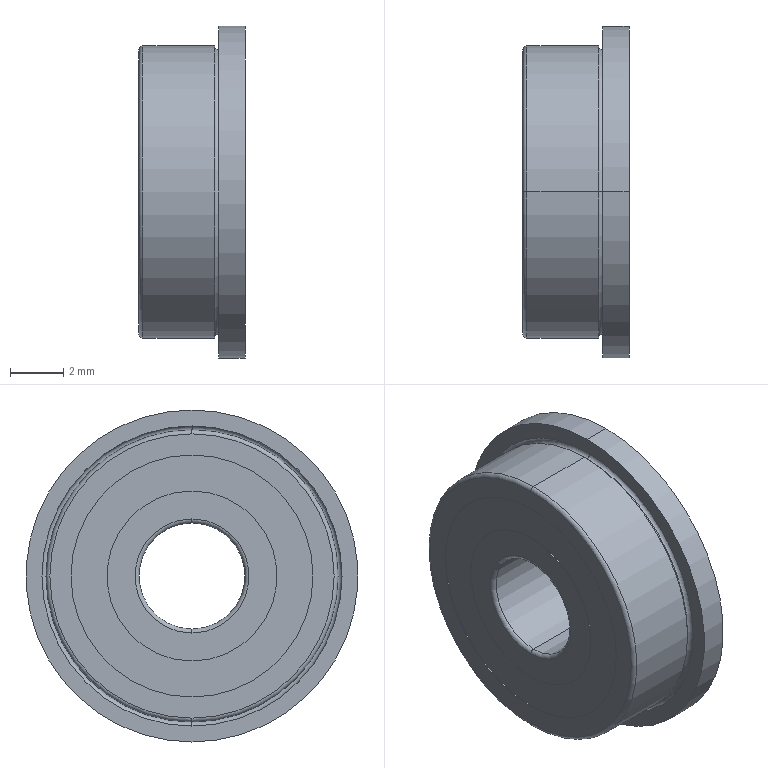Part | STEP file | 11-FL694ZZ11_FL694ZZ | 1 solid | 31 faces | box 4 x 12.5 x 12.5 mm | volume 353.722 mm3 | cylinder 14 | torus 10 | plane 7 | commonest cylinder face diameters 6.4 x4 9.11 x4 4 x2 11 x2 12.5 x2
STEP:
#1=CARTESIAN_POINT('',(2.85,0.,5.5));
#2=VERTEX_POINT('',#1);
#3=CARTESIAN_POINT('',(3.,0.,5.35));
#4=VERTEX_POINT('',#3);
#5=CARTESIAN_POINT('',(3.,0.,5.5));
#6=DIRECTION('',(0.,-1.,0.));
#7=DIRECTION('',(0.,0.,-1.));
#8=AXIS2_PLACEMENT_3D('',#5,#6,#7);
#9=CIRCLE('',#8,0.15);
#10=EDGE_CURVE('',#2,#4,#9,.T.);
#11=ORIENTED_EDGE('',*,*,#10,.T.);
#12=CARTESIAN_POINT('',(3.,0.,-5.35));
#13=VERTEX_POINT('',#12);
#14=CARTESIAN_POINT('',(3.,0.,0.));
#15=DIRECTION('',(-1.,0.,0.));
#16=DIRECTION('',(0.,0.,1.));
#17=AXIS2_PLACEMENT_3D('',#14,#15,#16);
#18=CIRCLE('',#17,5.35);
#19=EDGE_CURVE('',#4,#13,#18,.T.);
#20=ORIENTED_EDGE('',*,*,#19,.T.);
#21=CARTESIAN_POINT('',(2.85,0.,-5.5));
#22=VERTEX_POINT('',#21);
#23=CARTESIAN_POINT('',(3.,0.,-5.5));
#24=DIRECTION('',(0.,1.,0.));
#25=DIRECTION('',(0.,0.,1.));
#26=AXIS2_PLACEMENT_3D('',#23,#24,#25);
#27=CIRCLE('',#26,0.15);
#28=EDGE_CURVE('',#22,#13,#27,.T.);
#29=ORIENTED_EDGE('',*,*,#28,.F.);
#30=CARTESIAN_POINT('',(2.85,0.,0.));
#31=DIRECTION('',(-1.,0.,0.));
#32=DIRECTION('',(0.,0.,1.));
#33=AXIS2_PLACEMENT_3D('',#30,#31,#32);
#34=CIRCLE('',#33,5.5);
#35=EDGE_CURVE('',#2,#22,#34,.T.);
#36=ORIENTED_EDGE('',*,*,#35,.F.);
#37=EDGE_LOOP('',(#11,#20,#29,#36));
#38=FACE_OUTER_BOUND('',#37,.T.);
#39=CARTESIAN_POINT('',(3.,0.,0.));
#40=DIRECTION('',(-1.,0.,0.));
#41=DIRECTION('',(0.,0.,1.));
#42=AXIS2_PLACEMENT_3D('',#39,#40,#41);
#43=TOROIDAL_SURFACE('',#42,5.5,0.15);
#44=ADVANCED_FACE('',(#38),#43,.F.);
#45=ORIENTED_EDGE('',*,*,#28,.T.);
#46=CARTESIAN_POINT('',(3.,0.,0.));
#47=DIRECTION('',(-1.,0.,0.));
#48=DIRECTION('',(0.,0.,1.));
#49=AXIS2_PLACEMENT_3D('',#46,#47,#48);
#50=CIRCLE('',#49,5.35);
#51=EDGE_CURVE('',#13,#4,#50,.T.);
#52=ORIENTED_EDGE('',*,*,#51,.T.);
#53=ORIENTED_EDGE('',*,*,#10,.F.);
#54=CARTESIAN_POINT('',(2.85,0.,0.));
#55=DIRECTION('',(-1.,0.,0.));
#56=DIRECTION('',(0.,0.,1.));
#57=AXIS2_PLACEMENT_3D('',#54,#55,#56);
#58=CIRCLE('',#57,5.5);
#59=EDGE_CURVE('',#22,#2,#58,.T.);
#60=ORIENTED_EDGE('',*,*,#59,.F.);
#61=EDGE_LOOP('',(#45,#52,#53,#60));
#62=FACE_OUTER_BOUND('',#61,.T.);
#63=CARTESIAN_POINT('',(3.,0.,0.));
#64=DIRECTION('',(-1.,0.,0.));
#65=DIRECTION('',(0.,0.,1.));
#66=AXIS2_PLACEMENT_3D('',#63,#64,#65);
#67=TOROIDAL_SURFACE('',#66,5.5,0.15);
#68=ADVANCED_FACE('',(#62),#67,.F.);
#69=ORIENTED_EDGE('',*,*,#35,.T.);
#70=CARTESIAN_POINT('',(0.15,0.,-5.5));
#71=VERTEX_POINT('',#70);
#72=CARTESIAN_POINT('',(11.,0.,-5.5));
#73=DIRECTION('',(-1.,0.,0.));
#74=VECTOR('',#73,1000.);
#75=LINE('',#72,#74);
#76=EDGE_CURVE('',#22,#71,#75,.T.);
#77=ORIENTED_EDGE('',*,*,#76,.T.);
#78=CARTESIAN_POINT('',(0.15,0.,5.5));
#79=VERTEX_POINT('',#78);
#80=CARTESIAN_POINT('',(0.15,0.,0.));
#81=DIRECTION('',(-1.,0.,0.));
#82=DIRECTION('',(0.,0.,1.));
#83=AXIS2_PLACEMENT_3D('',#80,#81,#82);
#84=CIRCLE('',#83,5.5);
#85=EDGE_CURVE('',#79,#71,#84,.T.);
#86=ORIENTED_EDGE('',*,*,#85,.F.);
#87=CARTESIAN_POINT('',(11.,0.,5.5));
#88=DIRECTION('',(-1.,0.,0.));
#89=VECTOR('',#88,1000.);
#90=LINE('',#87,#89);
#91=EDGE_CURVE('',#2,#79,#90,.T.);
#92=ORIENTED_EDGE('',*,*,#91,.F.);
#93=EDGE_LOOP('',(#69,#77,#86,#92));
#94=FACE_OUTER_BOUND('',#93,.T.);
#95=CARTESIAN_POINT('',(11.,0.,0.));
#96=DIRECTION('',(-1.,0.,0.));
#97=DIRECTION('',(0.,0.,1.));
#98=AXIS2_PLACEMENT_3D('',#95,#96,#97);
#99=CYLINDRICAL_SURFACE('',#98,5.5);
#100=ADVANCED_FACE('',(#94),#99,.T.);
#101=ORIENTED_EDGE('',*,*,#51,.F.);
#102=CARTESIAN_POINT('',(3.,0.,-5.65));
#103=VERTEX_POINT('',#102);
#104=CARTESIAN_POINT('',(3.,0.,-5.5));
#105=DIRECTION('',(0.,1.,0.));
#106=DIRECTION('',(0.,0.,1.));
#107=AXIS2_PLACEMENT_3D('',#104,#105,#106);
#108=CIRCLE('',#107,0.15);
#109=EDGE_CURVE('',#13,#103,#108,.T.);
#110=ORIENTED_EDGE('',*,*,#109,.T.);
#111=CARTESIAN_POINT('',(3.,0.,5.65));
#112=VERTEX_POINT('',#111);
#113=CARTESIAN_POINT('',(3.,0.,0.));
#114=DIRECTION('',(-1.,0.,0.));
#115=DIRECTION('',(0.,0.,1.));
#116=AXIS2_PLACEMENT_3D('',#113,#114,#115);
#117=CIRCLE('',#116,5.65);
#118=EDGE_CURVE('',#103,#112,#117,.T.);
#119=ORIENTED_EDGE('',*,*,#118,.T.);
#120=CARTESIAN_POINT('',(3.,0.,5.5));
#121=DIRECTION('',(0.,-1.,0.));
#122=DIRECTION('',(0.,0.,-1.));
#123=AXIS2_PLACEMENT_3D('',#120,#121,#122);
#124=CIRCLE('',#123,0.15);
#125=EDGE_CURVE('',#4,#112,#124,.T.);
#126=ORIENTED_EDGE('',*,*,#125,.F.);
#127=EDGE_LOOP('',(#101,#110,#119,#126));
#128=FACE_OUTER_BOUND('',#127,.T.);
#129=CARTESIAN_POINT('',(3.,0.,0.));
#130=DIRECTION('',(-1.,0.,0.));
#131=DIRECTION('',(0.,0.,1.));
#132=AXIS2_PLACEMENT_3D('',#129,#130,#131);
#133=TOROIDAL_SURFACE('',#132,5.5,0.15);
#134=ADVANCED_FACE('',(#128),#133,.F.);
#135=CARTESIAN_POINT('',(4.,0.,6.25));
#136=VERTEX_POINT('',#135);
#137=CARTESIAN_POINT('',(4.,0.,-6.25));
#138=VERTEX_POINT('',#137);
#139=CARTESIAN_POINT('',(4.,0.,0.));
#140=DIRECTION('',(-1.,0.,0.));
#141=DIRECTION('',(0.,0.,1.));
#142=AXIS2_PLACEMENT_3D('',#139,#140,#141);
#143=CIRCLE('',#142,6.25);
#144=EDGE_CURVE('',#136,#138,#143,.T.);
#145=ORIENTED_EDGE('',*,*,#144,.T.);
#146=CARTESIAN_POINT('',(3.,0.,-6.25));
#147=VERTEX_POINT('',#146);
#148=CARTESIAN_POINT('',(11.,0.,-6.25));
#149=DIRECTION('',(-1.,0.,0.));
#150=VECTOR('',#149,1000.);
#151=LINE('',#148,#150);
#152=EDGE_CURVE('',#138,#147,#151,.T.);
#153=ORIENTED_EDGE('',*,*,#152,.T.);
#154=CARTESIAN_POINT('',(3.,0.,6.25));
#155=VERTEX_POINT('',#154);
#156=CARTESIAN_POINT('',(3.,0.,0.));
#157=DIRECTION('',(-1.,0.,0.));
#158=DIRECTION('',(0.,0.,1.));
#159=AXIS2_PLACEMENT_3D('',#156,#157,#158);
#160=CIRCLE('',#159,6.25);
#161=EDGE_CURVE('',#155,#147,#160,.T.);
#162=ORIENTED_EDGE('',*,*,#161,.F.);
#163=CARTESIAN_POINT('',(11.,0.,6.25));
#164=DIRECTION('',(-1.,0.,0.));
#165=VECTOR('',#164,1000.);
#166=LINE('',#163,#165);
#167=EDGE_CURVE('',#136,#155,#166,.T.);
#168=ORIENTED_EDGE('',*,*,#167,.F.);
#169=EDGE_LOOP('',(#145,#153,#162,#168));
#170=FACE_OUTER_BOUND('',#169,.T.);
#171=CARTESIAN_POINT('',(11.,0.,0.));
#172=DIRECTION('',(-1.,0.,0.));
#173=DIRECTION('',(0.,0.,1.));
#174=AXIS2_PLACEMENT_3D('',#171,#172,#173);
#175=CYLINDRICAL_SURFACE('',#174,6.25);
#176=ADVANCED_FACE('',(#170),#175,.T.);
#177=CARTESIAN_POINT('',(4.,0.,-4.555));
#178=VERTEX_POINT('',#177);
#179=CARTESIAN_POINT('',(4.,0.,4.555));
#180=VERTEX_POINT('',#179);
#181=CARTESIAN_POINT('',(4.,0.,0.));
#182=DIRECTION('',(-1.,0.,0.));
#183=DIRECTION('',(0.,0.,1.));
#184=AXIS2_PLACEMENT_3D('',#181,#182,#183);
#185=CIRCLE('',#184,4.555);
#186=EDGE_CURVE('',#178,#180,#185,.T.);
#187=ORIENTED_EDGE('',*,*,#186,.F.);
#188=CARTESIAN_POINT('',(3.974,0.,-4.555));
#189=VERTEX_POINT('',#188);
#190=CARTESIAN_POINT('',(11.,0.,-4.555));
#191=DIRECTION('',(-1.,0.,0.));
#192=VECTOR('',#191,1000.);
#193=LINE('',#190,#192);
#194=EDGE_CURVE('',#178,#189,#193,.T.);
#195=ORIENTED_EDGE('',*,*,#194,.T.);
#196=CARTESIAN_POINT('',(3.974,0.,4.555));
#197=VERTEX_POINT('',#196);
#198=CARTESIAN_POINT('',(3.974,0.,0.));
#199=DIRECTION('',(-1.,0.,0.));
#200=DIRECTION('',(0.,0.,1.));
#201=AXIS2_PLACEMENT_3D('',#198,#199,#200);
#202=CIRCLE('',#201,4.555);
#203=EDGE_CURVE('',#189,#197,#202,.T.);
#204=ORIENTED_EDGE('',*,*,#203,.T.);
#205=CARTESIAN_POINT('',(11.,0.,4.555));
#206=DIRECTION('',(-1.,0.,0.));
#207=VECTOR('',#206,1000.);
#208=LINE('',#205,#207);
#209=EDGE_CURVE('',#180,#197,#208,.T.);
#210=ORIENTED_EDGE('',*,*,#209,.F.);
#211=EDGE_LOOP('',(#187,#195,#204,#210));
#212=FACE_OUTER_BOUND('',#211,.T.);
#213=CARTESIAN_POINT('',(11.,0.,0.));
#214=DIRECTION('',(-1.,0.,0.));
#215=DIRECTION('',(0.,0.,1.));
#216=AXIS2_PLACEMENT_3D('',#213,#214,#215);
#217=CYLINDRICAL_SURFACE('',#216,4.555);
#218=ADVANCED_FACE('',(#212),#217,.F.);
#219=CARTESIAN_POINT('',(4.,0.,3.2));
#220=VERTEX_POINT('',#219);
#221=CARTESIAN_POINT('',(4.,0.,-3.2));
#222=VERTEX_POINT('',#221);
#223=CARTESIAN_POINT('',(4.,0.,0.));
#224=DIRECTION('',(-1.,0.,0.));
#225=DIRECTION('',(0.,0.,1.));
#226=AXIS2_PLACEMENT_3D('',#223,#224,#225);
#227=CIRCLE('',#226,3.2);
#228=EDGE_CURVE('',#220,#222,#227,.T.);
#229=ORIENTED_EDGE('',*,*,#228,.T.);
#230=CARTESIAN_POINT('',(3.974,0.,-3.2));
#231=VERTEX_POINT('',#230);
#232=CARTESIAN_POINT('',(11.,0.,-3.2));
#233=DIRECTION('',(-1.,0.,0.));
#234=VECTOR('',#233,1000.);
#235=LINE('',#232,#234);
#236=EDGE_CURVE('',#222,#231,#235,.T.);
#237=ORIENTED_EDGE('',*,*,#236,.T.);
#238=CARTESIAN_POINT('',(3.974,0.,3.2));
#239=VERTEX_POINT('',#238);
#240=CARTESIAN_POINT('',(3.974,0.,0.));
#241=DIRECTION('',(-1.,0.,0.));
#242=DIRECTION('',(0.,0.,1.));
#243=AXIS2_PLACEMENT_3D('',#240,#241,#242);
#244=CIRCLE('',#243,3.2);
#245=EDGE_CURVE('',#239,#231,#244,.T.);
#246=ORIENTED_EDGE('',*,*,#245,.F.);
#247=CARTESIAN_POINT('',(11.,0.,3.2));
#248=DIRECTION('',(-1.,0.,0.));
#249=VECTOR('',#248,1000.);
#250=LINE('',#247,#249);
#251=EDGE_CURVE('',#220,#239,#250,.T.);
#252=ORIENTED_EDGE('',*,*,#251,.F.);
#253=EDGE_LOOP('',(#229,#237,#246,#252));
#254=FACE_OUTER_BOUND('',#253,.T.);
#255=CARTESIAN_POINT('',(11.,0.,0.));
#256=DIRECTION('',(-1.,0.,0.));
#257=DIRECTION('',(0.,0.,1.));
#258=AXIS2_PLACEMENT_3D('',#255,#256,#257);
#259=CYLINDRICAL_SURFACE('',#258,3.2);
#260=ADVANCED_FACE('',(#254),#259,.T.);
#261=CARTESIAN_POINT('',(3.85,0.,2.));
#262=VERTEX_POINT('',#261);
#263=CARTESIAN_POINT('',(3.85,0.,-2.));
#264=VERTEX_POINT('',#263);
#265=CARTESIAN_POINT('',(3.85,0.,0.));
#266=DIRECTION('',(-1.,0.,0.));
#267=DIRECTION('',(0.,0.,1.));
#268=AXIS2_PLACEMENT_3D('',#265,#266,#267);
#269=CIRCLE('',#268,2.);
#270=EDGE_CURVE('',#262,#264,#269,.T.);
#271=ORIENTED_EDGE('',*,*,#270,.T.);
#272=CARTESIAN_POINT('',(4.,0.,-2.15));
#273=VERTEX_POINT('',#272);
#274=CARTESIAN_POINT('',(3.85,0.,-2.15));
#275=DIRECTION('',(0.,1.,0.));
#276=DIRECTION('',(0.,0.,1.));
#277=AXIS2_PLACEMENT_3D('',#274,#275,#276);
#278=CIRCLE('',#277,0.15);
#279=EDGE_CURVE('',#264,#273,#278,.T.);
#280=ORIENTED_EDGE('',*,*,#279,.T.);
#281=CARTESIAN_POINT('',(4.,0.,2.15));
#282=VERTEX_POINT('',#281);
#283=CARTESIAN_POINT('',(4.,0.,0.));
#284=DIRECTION('',(-1.,0.,0.));
#285=DIRECTION('',(0.,0.,1.));
#286=AXIS2_PLACEMENT_3D('',#283,#284,#285);
#287=CIRCLE('',#286,2.15);
#288=EDGE_CURVE('',#282,#273,#287,.T.);
#289=ORIENTED_EDGE('',*,*,#288,.F.);
#290=CARTESIAN_POINT('',(3.85,0.,2.15));
#291=DIRECTION('',(0.,-1.,0.));
#292=DIRECTION('',(0.,0.,-1.));
#293=AXIS2_PLACEMENT_3D('',#290,#291,#292);
#294=CIRCLE('',#293,0.15);
#295=EDGE_CURVE('',#262,#282,#294,.T.);
#296=ORIENTED_EDGE('',*,*,#295,.F.);
#297=EDGE_LOOP('',(#271,#280,#289,#296));
#298=FACE_OUTER_BOUND('',#297,.T.);
#299=CARTESIAN_POINT('',(3.85,0.,0.));
#300=DIRECTION('',(-1.,0.,0.));
#301=DIRECTION('',(0.,0.,1.));
#302=AXIS2_PLACEMENT_3D('',#299,#300,#301);
#303=TOROIDAL_SURFACE('',#302,2.15,0.15);
#304=ADVANCED_FACE('',(#298),#303,.T.);
#305=CARTESIAN_POINT('',(3.85,0.,0.));
#306=DIRECTION('',(-1.,0.,0.));
#307=DIRECTION('',(0.,0.,1.));
#308=AXIS2_PLACEMENT_3D('',#305,#306,#307);
#309=CIRCLE('',#308,2.);
#310=EDGE_CURVE('',#264,#262,#309,.T.);
#311=ORIENTED_EDGE('',*,*,#310,.F.);
#312=CARTESIAN_POINT('',(0.15,0.,-2.));
#313=VERTEX_POINT('',#312);
#314=CARTESIAN_POINT('',(11.,0.,-2.));
#315=DIRECTION('',(-1.,0.,0.));
#316=VECTOR('',#315,1000.);
#317=LINE('',#314,#316);
#318=EDGE_CURVE('',#264,#313,#317,.T.);
#319=ORIENTED_EDGE('',*,*,#318,.T.);
#320=CARTESIAN_POINT('',(0.15,0.,2.));
#321=VERTEX_POINT('',#320);
#322=CARTESIAN_POINT('',(0.15,0.,0.));
#323=DIRECTION('',(-1.,0.,0.));
#324=DIRECTION('',(0.,0.,1.));
#325=AXIS2_PLACEMENT_3D('',#322,#323,#324);
#326=CIRCLE('',#325,2.);
#327=EDGE_CURVE('',#313,#321,#326,.T.);
#328=ORIENTED_EDGE('',*,*,#327,.T.);
#329=CARTESIAN_POINT('',(11.,0.,2.));
#330=DIRECTION('',(-1.,0.,0.));
#331=VECTOR('',#330,1000.);
#332=LINE('',#329,#331);
#333=EDGE_CURVE('',#262,#321,#332,.T.);
#334=ORIENTED_EDGE('',*,*,#333,.F.);
#335=EDGE_LOOP('',(#311,#319,#328,#334));
#336=FACE_OUTER_BOUND('',#335,.T.);
#337=CARTESIAN_POINT('',(11.,0.,0.));
#338=DIRECTION('',(-1.,0.,0.));
#339=DIRECTION('',(0.,0.,1.));
#340=AXIS2_PLACEMENT_3D('',#337,#338,#339);
#341=CYLINDRICAL_SURFACE('',#340,2.);
#342=ADVANCED_FACE('',(#336),#341,.F.);
#343=CARTESIAN_POINT('',(0.,0.,2.15));
#344=VERTEX_POINT('',#343);
#345=CARTESIAN_POINT('',(0.,0.,-2.15));
#346=VERTEX_POINT('',#345);
#347=CARTESIAN_POINT('',(0.,0.,0.));
#348=DIRECTION('',(-1.,0.,0.));
#349=DIRECTION('',(0.,0.,1.));
#350=AXIS2_PLACEMENT_3D('',#347,#348,#349);
#351=CIRCLE('',#350,2.15);
#352=EDGE_CURVE('',#344,#346,#351,.T.);
#353=ORIENTED_EDGE('',*,*,#352,.T.);
#354=CARTESIAN_POINT('',(0.15,0.,-2.15));
#355=DIRECTION('',(0.,1.,0.));
#356=DIRECTION('',(0.,0.,1.));
#357=AXIS2_PLACEMENT_3D('',#354,#355,#356);
#358=CIRCLE('',#357,0.15);
#359=EDGE_CURVE('',#346,#313,#358,.T.);
#360=ORIENTED_EDGE('',*,*,#359,.T.);
#361=CARTESIAN_POINT('',(0.15,0.,0.));
#362=DIRECTION('',(-1.,0.,0.));
#363=DIRECTION('',(0.,0.,1.));
#364=AXIS2_PLACEMENT_3D('',#361,#362,#363);
#365=CIRCLE('',#364,2.);
#366=EDGE_CURVE('',#321,#313,#365,.T.);
#367=ORIENTED_EDGE('',*,*,#366,.F.);
#368=CARTESIAN_POINT('',(0.15,0.,2.15));
#369=DIRECTION('',(0.,-1.,0.));
#370=DIRECTION('',(0.,0.,-1.));
#371=AXIS2_PLACEMENT_3D('',#368,#369,#370);
#372=CIRCLE('',#371,0.15);
#373=EDGE_CURVE('',#344,#321,#372,.T.);
#374=ORIENTED_EDGE('',*,*,#373,.F.);
#375=EDGE_LOOP('',(#353,#360,#367,#374));
#376=FACE_OUTER_BOUND('',#375,.T.);
#377=CARTESIAN_POINT('',(0.15,0.,0.));
#378=DIRECTION('',(-1.,0.,0.));
#379=DIRECTION('',(0.,0.,1.));
#380=AXIS2_PLACEMENT_3D('',#377,#378,#379);
#381=TOROIDAL_SURFACE('',#380,2.15,0.15);
#382=ADVANCED_FACE('',(#376),#381,.T.);
#383=CARTESIAN_POINT('',(0.026,0.,3.2));
#384=VERTEX_POINT('',#383);
#385=CARTESIAN_POINT('',(0.026,0.,-3.2));
#386=VERTEX_POINT('',#385);
#387=CARTESIAN_POINT('',(0.026,0.,0.));
#388=DIRECTION('',(-1.,0.,0.));
#389=DIRECTION('',(0.,0.,1.));
#390=AXIS2_PLACEMENT_3D('',#387,#388,#389);
#391=CIRCLE('',#390,3.2);
#392=EDGE_CURVE('',#384,#386,#391,.T.);
#393=ORIENTED_EDGE('',*,*,#392,.T.);
#394=CARTESIAN_POINT('',(0.,0.,-3.2));
#395=VERTEX_POINT('',#394);
#396=CARTESIAN_POINT('',(11.,0.,-3.2));
#397=DIRECTION('',(-1.,0.,0.));
#398=VECTOR('',#397,1000.);
#399=LINE('',#396,#398);
#400=EDGE_CURVE('',#386,#395,#399,.T.);
#401=ORIENTED_EDGE('',*,*,#400,.T.);
#402=CARTESIAN_POINT('',(0.,0.,3.2));
#403=VERTEX_POINT('',#402);
#404=CARTESIAN_POINT('',(0.,0.,0.));
#405=DIRECTION('',(-1.,0.,0.));
#406=DIRECTION('',(0.,0.,1.));
#407=AXIS2_PLACEMENT_3D('',#404,#405,#406);
#408=CIRCLE('',#407,3.2);
#409=EDGE_CURVE('',#403,#395,#408,.T.);
#410=ORIENTED_EDGE('',*,*,#409,.F.);
#411=CARTESIAN_POINT('',(11.,0.,3.2));
#412=DIRECTION('',(-1.,0.,0.));
#413=VECTOR('',#412,1000.);
#414=LINE('',#411,#413);
#415=EDGE_CURVE('',#384,#403,#414,.T.);
#416=ORIENTED_EDGE('',*,*,#415,.F.);
#417=EDGE_LOOP('',(#393,#401,#410,#416));
#418=FACE_OUTER_BOUND('',#417,.T.);
#419=CARTESIAN_POINT('',(11.,0.,0.));
#420=DIRECTION('',(-1.,0.,0.));
#421=DIRECTION('',(0.,0.,1.));
#422=AXIS2_PLACEMENT_3D('',#419,#420,#421);
#423=CYLINDRICAL_SURFACE('',#422,3.2);
#424=ADVANCED_FACE('',(#418),#423,.T.);
#425=CARTESIAN_POINT('',(0.026,0.,-4.555));
#426=VERTEX_POINT('',#425);
#427=CARTESIAN_POINT('',(0.026,0.,4.555));
#428=VERTEX_POINT('',#427);
#429=CARTESIAN_POINT('',(0.026,0.,0.));
#430=DIRECTION('',(-1.,0.,0.));
#431=DIRECTION('',(0.,0.,1.));
#432=AXIS2_PLACEMENT_3D('',#429,#430,#431);
#433=CIRCLE('',#432,4.555);
#434=EDGE_CURVE('',#426,#428,#433,.T.);
#435=ORIENTED_EDGE('',*,*,#434,.F.);
#436=CARTESIAN_POINT('',(0.,0.,-4.555));
#437=VERTEX_POINT('',#436);
#438=CARTESIAN_POINT('',(11.,0.,-4.555));
#439=DIRECTION('',(-1.,0.,0.));
#440=VECTOR('',#439,1000.);
#441=LINE('',#438,#440);
#442=EDGE_CURVE('',#426,#437,#441,.T.);
#443=ORIENTED_EDGE('',*,*,#442,.T.);
#444=CARTESIAN_POINT('',(0.,0.,4.555));
#445=VERTEX_POINT('',#444);
#446=CARTESIAN_POINT('',(0.,0.,0.));
#447=DIRECTION('',(-1.,0.,0.));
#448=DIRECTION('',(0.,0.,1.));
#449=AXIS2_PLACEMENT_3D('',#446,#447,#448);
#450=CIRCLE('',#449,4.555);
#451=EDGE_CURVE('',#437,#445,#450,.T.);
#452=ORIENTED_EDGE('',*,*,#451,.T.);
#453=CARTESIAN_POINT('',(11.,0.,4.555));
#454=DIRECTION('',(-1.,0.,0.));
#455=VECTOR('',#454,1000.);
#456=LINE('',#453,#455);
#457=EDGE_CURVE('',#428,#445,#456,.T.);
#458=ORIENTED_EDGE('',*,*,#457,.F.);
#459=EDGE_LOOP('',(#435,#443,#452,#458));
#460=FACE_OUTER_BOUND('',#459,.T.);
#461=CARTESIAN_POINT('',(11.,0.,0.));
#462=DIRECTION('',(-1.,0.,0.));
#463=DIRECTION('',(0.,0.,1.));
#464=AXIS2_PLACEMENT_3D('',#461,#462,#463);
#465=CYLINDRICAL_SURFACE('',#464,4.555);
#466=ADVANCED_FACE('',(#460),#465,.F.);
#467=ORIENTED_EDGE('',*,*,#85,.T.);
#468=CARTESIAN_POINT('',(0.,0.,-5.35));
#469=VERTEX_POINT('',#468);
#470=CARTESIAN_POINT('',(0.15,0.,-5.35));
#471=DIRECTION('',(0.,1.,0.));
#472=DIRECTION('',(0.,0.,1.));
#473=AXIS2_PLACEMENT_3D('',#470,#471,#472);
#474=CIRCLE('',#473,0.15);
#475=EDGE_CURVE('',#71,#469,#474,.T.);
#476=ORIENTED_EDGE('',*,*,#475,.T.);
#477=CARTESIAN_POINT('',(0.,0.,5.35));
#478=VERTEX_POINT('',#477);
#479=CARTESIAN_POINT('',(0.,0.,0.));
#480=DIRECTION('',(-1.,0.,0.));
#481=DIRECTION('',(0.,0.,1.));
#482=AXIS2_PLACEMENT_3D('',#479,#480,#481);
#483=CIRCLE('',#482,5.35);
#484=EDGE_CURVE('',#478,#469,#483,.T.);
#485=ORIENTED_EDGE('',*,*,#484,.F.);
#486=CARTESIAN_POINT('',(0.15,0.,5.35));
#487=DIRECTION('',(0.,-1.,0.));
#488=DIRECTION('',(0.,0.,-1.));
#489=AXIS2_PLACEMENT_3D('',#486,#487,#488);
#490=CIRCLE('',#489,0.15);
#491=EDGE_CURVE('',#79,#478,#490,.T.);
#492=ORIENTED_EDGE('',*,*,#491,.F.);
#493=EDGE_LOOP('',(#467,#476,#485,#492));
#494=FACE_OUTER_BOUND('',#493,.T.);
#495=CARTESIAN_POINT('',(0.15,0.,0.));
#496=DIRECTION('',(-1.,0.,0.));
#497=DIRECTION('',(0.,0.,1.));
#498=AXIS2_PLACEMENT_3D('',#495,#496,#497);
#499=TOROIDAL_SURFACE('',#498,5.35,0.15);
#500=ADVANCED_FACE('',(#494),#499,.T.);
#501=ORIENTED_EDGE('',*,*,#475,.F.);
#502=CARTESIAN_POINT('',(0.15,0.,0.));
#503=DIRECTION('',(-1.,0.,0.));
#504=DIRECTION('',(0.,0.,1.));
#505=AXIS2_PLACEMENT_3D('',#502,#503,#504);
#506=CIRCLE('',#505,5.5);
#507=EDGE_CURVE('',#71,#79,#506,.T.);
#508=ORIENTED_EDGE('',*,*,#507,.T.);
#509=ORIENTED_EDGE('',*,*,#491,.T.);
#510=CARTESIAN_POINT('',(0.,0.,0.));
#511=DIRECTION('',(-1.,0.,0.));
#512=DIRECTION('',(0.,0.,1.));
#513=AXIS2_PLACEMENT_3D('',#510,#511,#512);
#514=CIRCLE('',#513,5.35);
#515=EDGE_CURVE('',#469,#478,#514,.T.);
#516=ORIENTED_EDGE('',*,*,#515,.F.);
#517=EDGE_LOOP('',(#501,#508,#509,#516));
#518=FACE_OUTER_BOUND('',#517,.T.);
#519=CARTESIAN_POINT('',(0.15,0.,0.));
#520=DIRECTION('',(-1.,0.,0.));
#521=DIRECTION('',(0.,0.,1.));
#522=AXIS2_PLACEMENT_3D('',#519,#520,#521);
#523=TOROIDAL_SURFACE('',#522,5.35,0.15);
#524=ADVANCED_FACE('',(#518),#523,.T.);
#525=CARTESIAN_POINT('',(0.,0.,0.));
#526=DIRECTION('',(-1.,0.,0.));
#527=DIRECTION('',(0.,0.,1.));
#528=AXIS2_PLACEMENT_3D('',#525,#526,#527);
#529=CIRCLE('',#528,4.555);
#530=EDGE_CURVE('',#445,#437,#529,.T.);
#531=ORIENTED_EDGE('',*,*,#530,.F.);
#532=ORIENTED_EDGE('',*,*,#451,.F.);
#533=EDGE_LOOP('',(#531,#532));
#534=FACE_BOUND('',#533,.T.);
#535=ORIENTED_EDGE('',*,*,#484,.T.);
#536=ORIENTED_EDGE('',*,*,#515,.T.);
#537=EDGE_LOOP('',(#535,#536));
#538=FACE_OUTER_BOUND('',#537,.T.);
#539=CARTESIAN_POINT('',(0.,5.35,0.));
#540=DIRECTION('',(1.,0.,0.));
#541=DIRECTION('',(0.,0.,-1.));
#542=AXIS2_PLACEMENT_3D('',#539,#540,#541);
#543=PLANE('',#542);
#544=ADVANCED_FACE('',(#534,#538),#543,.F.);
#545=ORIENTED_EDGE('',*,*,#442,.F.);
#546=CARTESIAN_POINT('',(0.026,0.,0.));
#547=DIRECTION('',(-1.,0.,0.));
#548=DIRECTION('',(0.,0.,1.));
#549=AXIS2_PLACEMENT_3D('',#546,#547,#548);
#550=CIRCLE('',#549,4.555);
#551=EDGE_CURVE('',#428,#426,#550,.T.);
#552=ORIENTED_EDGE('',*,*,#551,.F.);
#553=ORIENTED_EDGE('',*,*,#457,.T.);
#554=ORIENTED_EDGE('',*,*,#530,.T.);
#555=EDGE_LOOP('',(#545,#552,#553,#554));
#556=FACE_OUTER_BOUND('',#555,.T.);
#557=CARTESIAN_POINT('',(11.,0.,0.));
#558=DIRECTION('',(-1.,0.,0.));
#559=DIRECTION('',(0.,0.,1.));
#560=AXIS2_PLACEMENT_3D('',#557,#558,#559);
#561=CYLINDRICAL_SURFACE('',#560,4.555);
#562=ADVANCED_FACE('',(#556),#561,.F.);
#563=ORIENTED_EDGE('',*,*,#392,.F.);
#564=CARTESIAN_POINT('',(0.026,0.,0.));
#565=DIRECTION('',(-1.,0.,0.));
#566=DIRECTION('',(0.,0.,1.));
#567=AXIS2_PLACEMENT_3D('',#564,#565,#566);
#568=CIRCLE('',#567,3.2);
#569=EDGE_CURVE('',#386,#384,#568,.T.);
#570=ORIENTED_EDGE('',*,*,#569,.F.);
#571=EDGE_LOOP('',(#563,#570));
#572=FACE_BOUND('',#571,.T.);
#573=ORIENTED_EDGE('',*,*,#551,.T.);
#574=ORIENTED_EDGE('',*,*,#434,.T.);
#575=EDGE_LOOP('',(#573,#574));
#576=FACE_OUTER_BOUND('',#575,.T.);
#577=CARTESIAN_POINT('',(0.026,4.555,0.));
#578=DIRECTION('',(1.,0.,0.));
#579=DIRECTION('',(0.,0.,-1.));
#580=AXIS2_PLACEMENT_3D('',#577,#578,#579);
#581=PLANE('',#580);
#582=ADVANCED_FACE('',(#572,#576),#581,.F.);
#583=ORIENTED_EDGE('',*,*,#400,.F.);
#584=ORIENTED_EDGE('',*,*,#569,.T.);
#585=ORIENTED_EDGE('',*,*,#415,.T.);
#586=CARTESIAN_POINT('',(0.,0.,0.));
#587=DIRECTION('',(-1.,0.,0.));
#588=DIRECTION('',(0.,0.,1.));
#589=AXIS2_PLACEMENT_3D('',#586,#587,#588);
#590=CIRCLE('',#589,3.2);
#591=EDGE_CURVE('',#395,#403,#590,.T.);
#592=ORIENTED_EDGE('',*,*,#591,.F.);
#593=EDGE_LOOP('',(#583,#584,#585,#592));
#594=FACE_OUTER_BOUND('',#593,.T.);
#595=CARTESIAN_POINT('',(11.,0.,0.));
#596=DIRECTION('',(-1.,0.,0.));
#597=DIRECTION('',(0.,0.,1.));
#598=AXIS2_PLACEMENT_3D('',#595,#596,#597);
#599=CYLINDRICAL_SURFACE('',#598,3.2);
#600=ADVANCED_FACE('',(#594),#599,.T.);
#601=ORIENTED_EDGE('',*,*,#352,.F.);
#602=CARTESIAN_POINT('',(0.,0.,0.));
#603=DIRECTION('',(-1.,0.,0.));
#604=DIRECTION('',(0.,0.,1.));
#605=AXIS2_PLACEMENT_3D('',#602,#603,#604);
#606=CIRCLE('',#605,2.15);
#607=EDGE_CURVE('',#346,#344,#606,.T.);
#608=ORIENTED_EDGE('',*,*,#607,.F.);
#609=EDGE_LOOP('',(#601,#608));
#610=FACE_BOUND('',#609,.T.);
#611=ORIENTED_EDGE('',*,*,#409,.T.);
#612=ORIENTED_EDGE('',*,*,#591,.T.);
#613=EDGE_LOOP('',(#611,#612));
#614=FACE_OUTER_BOUND('',#613,.T.);
#615=CARTESIAN_POINT('',(0.,3.2,0.));
#616=DIRECTION('',(1.,0.,0.));
#617=DIRECTION('',(0.,0.,-1.));
#618=AXIS2_PLACEMENT_3D('',#615,#616,#617);
#619=PLANE('',#618);
#620=ADVANCED_FACE('',(#610,#614),#619,.F.);
#621=ORIENTED_EDGE('',*,*,#359,.F.);
#622=ORIENTED_EDGE('',*,*,#607,.T.);
#623=ORIENTED_EDGE('',*,*,#373,.T.);
#624=ORIENTED_EDGE('',*,*,#327,.F.);
#625=EDGE_LOOP('',(#621,#622,#623,#624));
#626=FACE_OUTER_BOUND('',#625,.T.);
#627=CARTESIAN_POINT('',(0.15,0.,0.));
#628=DIRECTION('',(-1.,0.,0.));
#629=DIRECTION('',(0.,0.,1.));
#630=AXIS2_PLACEMENT_3D('',#627,#628,#629);
#631=TOROIDAL_SURFACE('',#630,2.15,0.15);
#632=ADVANCED_FACE('',(#626),#631,.T.);
#633=ORIENTED_EDGE('',*,*,#318,.F.);
#634=ORIENTED_EDGE('',*,*,#270,.F.);
#635=ORIENTED_EDGE('',*,*,#333,.T.);
#636=ORIENTED_EDGE('',*,*,#366,.T.);
#637=EDGE_LOOP('',(#633,#634,#635,#636));
#638=FACE_OUTER_BOUND('',#637,.T.);
#639=CARTESIAN_POINT('',(11.,0.,0.));
#640=DIRECTION('',(-1.,0.,0.));
#641=DIRECTION('',(0.,0.,1.));
#642=AXIS2_PLACEMENT_3D('',#639,#640,#641);
#643=CYLINDRICAL_SURFACE('',#642,2.);
#644=ADVANCED_FACE('',(#638),#643,.F.);
#645=ORIENTED_EDGE('',*,*,#279,.F.);
#646=ORIENTED_EDGE('',*,*,#310,.T.);
#647=ORIENTED_EDGE('',*,*,#295,.T.);
#648=CARTESIAN_POINT('',(4.,0.,0.));
#649=DIRECTION('',(-1.,0.,0.));
#650=DIRECTION('',(0.,0.,1.));
#651=AXIS2_PLACEMENT_3D('',#648,#649,#650);
#652=CIRCLE('',#651,2.15);
#653=EDGE_CURVE('',#273,#282,#652,.T.);
#654=ORIENTED_EDGE('',*,*,#653,.F.);
#655=EDGE_LOOP('',(#645,#646,#647,#654));
#656=FACE_OUTER_BOUND('',#655,.T.);
#657=CARTESIAN_POINT('',(3.85,0.,0.));
#658=DIRECTION('',(-1.,0.,0.));
#659=DIRECTION('',(0.,0.,1.));
#660=AXIS2_PLACEMENT_3D('',#657,#658,#659);
#661=TOROIDAL_SURFACE('',#660,2.15,0.15);
#662=ADVANCED_FACE('',(#656),#661,.T.);
#663=ORIENTED_EDGE('',*,*,#228,.F.);
#664=CARTESIAN_POINT('',(4.,0.,0.));
#665=DIRECTION('',(-1.,0.,0.));
#666=DIRECTION('',(0.,0.,1.));
#667=AXIS2_PLACEMENT_3D('',#664,#665,#666);
#668=CIRCLE('',#667,3.2);
#669=EDGE_CURVE('',#222,#220,#668,.T.);
#670=ORIENTED_EDGE('',*,*,#669,.F.);
#671=EDGE_LOOP('',(#663,#670));
#672=FACE_OUTER_BOUND('',#671,.T.);
#673=ORIENTED_EDGE('',*,*,#288,.T.);
#674=ORIENTED_EDGE('',*,*,#653,.T.);
#675=EDGE_LOOP('',(#673,#674));
#676=FACE_BOUND('',#675,.T.);
#677=CARTESIAN_POINT('',(4.,2.15,0.));
#678=DIRECTION('',(-1.,0.,0.));
#679=DIRECTION('',(0.,0.,1.));
#680=AXIS2_PLACEMENT_3D('',#677,#678,#679);
#681=PLANE('',#680);
#682=ADVANCED_FACE('',(#672,#676),#681,.F.);
#683=ORIENTED_EDGE('',*,*,#236,.F.);
#684=ORIENTED_EDGE('',*,*,#669,.T.);
#685=ORIENTED_EDGE('',*,*,#251,.T.);
#686=CARTESIAN_POINT('',(3.974,0.,0.));
#687=DIRECTION('',(-1.,0.,0.));
#688=DIRECTION('',(0.,0.,1.));
#689=AXIS2_PLACEMENT_3D('',#686,#687,#688);
#690=CIRCLE('',#689,3.2);
#691=EDGE_CURVE('',#231,#239,#690,.T.);
#692=ORIENTED_EDGE('',*,*,#691,.F.);
#693=EDGE_LOOP('',(#683,#684,#685,#692));
#694=FACE_OUTER_BOUND('',#693,.T.);
#695=CARTESIAN_POINT('',(11.,0.,0.));
#696=DIRECTION('',(-1.,0.,0.));
#697=DIRECTION('',(0.,0.,1.));
#698=AXIS2_PLACEMENT_3D('',#695,#696,#697);
#699=CYLINDRICAL_SURFACE('',#698,3.2);
#700=ADVANCED_FACE('',(#694),#699,.T.);
#701=CARTESIAN_POINT('',(3.974,0.,0.));
#702=DIRECTION('',(-1.,0.,0.));
#703=DIRECTION('',(0.,0.,1.));
#704=AXIS2_PLACEMENT_3D('',#701,#702,#703);
#705=CIRCLE('',#704,4.555);
#706=EDGE_CURVE('',#197,#189,#705,.T.);
#707=ORIENTED_EDGE('',*,*,#706,.F.);
#708=ORIENTED_EDGE('',*,*,#203,.F.);
#709=EDGE_LOOP('',(#707,#708));
#710=FACE_OUTER_BOUND('',#709,.T.);
#711=ORIENTED_EDGE('',*,*,#245,.T.);
#712=ORIENTED_EDGE('',*,*,#691,.T.);
#713=EDGE_LOOP('',(#711,#712));
#714=FACE_BOUND('',#713,.T.);
#715=CARTESIAN_POINT('',(3.974,3.2,0.));
#716=DIRECTION('',(-1.,0.,0.));
#717=DIRECTION('',(0.,0.,1.));
#718=AXIS2_PLACEMENT_3D('',#715,#716,#717);
#719=PLANE('',#718);
#720=ADVANCED_FACE('',(#710,#714),#719,.F.);
#721=ORIENTED_EDGE('',*,*,#194,.F.);
#722=CARTESIAN_POINT('',(4.,0.,0.));
#723=DIRECTION('',(-1.,0.,0.));
#724=DIRECTION('',(0.,0.,1.));
#725=AXIS2_PLACEMENT_3D('',#722,#723,#724);
#726=CIRCLE('',#725,4.555);
#727=EDGE_CURVE('',#180,#178,#726,.T.);
#728=ORIENTED_EDGE('',*,*,#727,.F.);
#729=ORIENTED_EDGE('',*,*,#209,.T.);
#730=ORIENTED_EDGE('',*,*,#706,.T.);
#731=EDGE_LOOP('',(#721,#728,#729,#730));
#732=FACE_OUTER_BOUND('',#731,.T.);
#733=CARTESIAN_POINT('',(11.,0.,0.));
#734=DIRECTION('',(-1.,0.,0.));
#735=DIRECTION('',(0.,0.,1.));
#736=AXIS2_PLACEMENT_3D('',#733,#734,#735);
#737=CYLINDRICAL_SURFACE('',#736,4.555);
#738=ADVANCED_FACE('',(#732),#737,.F.);
#739=ORIENTED_EDGE('',*,*,#144,.F.);
#740=CARTESIAN_POINT('',(4.,0.,0.));
#741=DIRECTION('',(-1.,0.,0.));
#742=DIRECTION('',(0.,0.,1.));
#743=AXIS2_PLACEMENT_3D('',#740,#741,#742);
#744=CIRCLE('',#743,6.25);
#745=EDGE_CURVE('',#138,#136,#744,.T.);
#746=ORIENTED_EDGE('',*,*,#745,.F.);
#747=EDGE_LOOP('',(#739,#746));
#748=FACE_OUTER_BOUND('',#747,.T.);
#749=ORIENTED_EDGE('',*,*,#727,.T.);
#750=ORIENTED_EDGE('',*,*,#186,.T.);
#751=EDGE_LOOP('',(#749,#750));
#752=FACE_BOUND('',#751,.T.);
#753=CARTESIAN_POINT('',(4.,4.555,0.));
#754=DIRECTION('',(-1.,0.,0.));
#755=DIRECTION('',(0.,0.,1.));
#756=AXIS2_PLACEMENT_3D('',#753,#754,#755);
#757=PLANE('',#756);
#758=ADVANCED_FACE('',(#748,#752),#757,.F.);
#759=ORIENTED_EDGE('',*,*,#152,.F.);
#760=ORIENTED_EDGE('',*,*,#745,.T.);
#761=ORIENTED_EDGE('',*,*,#167,.T.);
#762=CARTESIAN_POINT('',(3.,0.,0.));
#763=DIRECTION('',(-1.,0.,0.));
#764=DIRECTION('',(0.,0.,1.));
#765=AXIS2_PLACEMENT_3D('',#762,#763,#764);
#766=CIRCLE('',#765,6.25);
#767=EDGE_CURVE('',#147,#155,#766,.T.);
#768=ORIENTED_EDGE('',*,*,#767,.F.);
#769=EDGE_LOOP('',(#759,#760,#761,#768));
#770=FACE_OUTER_BOUND('',#769,.T.);
#771=CARTESIAN_POINT('',(11.,0.,0.));
#772=DIRECTION('',(-1.,0.,0.));
#773=DIRECTION('',(0.,0.,1.));
#774=AXIS2_PLACEMENT_3D('',#771,#772,#773);
#775=CYLINDRICAL_SURFACE('',#774,6.25);
#776=ADVANCED_FACE('',(#770),#775,.T.);
#777=CARTESIAN_POINT('',(3.,0.,0.));
#778=DIRECTION('',(-1.,0.,0.));
#779=DIRECTION('',(0.,0.,1.));
#780=AXIS2_PLACEMENT_3D('',#777,#778,#779);
#781=CIRCLE('',#780,5.65);
#782=EDGE_CURVE('',#112,#103,#781,.T.);
#783=ORIENTED_EDGE('',*,*,#782,.F.);
#784=ORIENTED_EDGE('',*,*,#118,.F.);
#785=EDGE_LOOP('',(#783,#784));
#786=FACE_BOUND('',#785,.T.);
#787=ORIENTED_EDGE('',*,*,#161,.T.);
#788=ORIENTED_EDGE('',*,*,#767,.T.);
#789=EDGE_LOOP('',(#787,#788));
#790=FACE_OUTER_BOUND('',#789,.T.);
#791=CARTESIAN_POINT('',(3.,6.25,0.));
#792=DIRECTION('',(1.,0.,0.));
#793=DIRECTION('',(0.,0.,-1.));
#794=AXIS2_PLACEMENT_3D('',#791,#792,#793);
#795=PLANE('',#794);
#796=ADVANCED_FACE('',(#786,#790),#795,.F.);
#797=ORIENTED_EDGE('',*,*,#19,.F.);
#798=ORIENTED_EDGE('',*,*,#125,.T.);
#799=ORIENTED_EDGE('',*,*,#782,.T.);
#800=ORIENTED_EDGE('',*,*,#109,.F.);
#801=EDGE_LOOP('',(#797,#798,#799,#800));
#802=FACE_OUTER_BOUND('',#801,.T.);
#803=CARTESIAN_POINT('',(3.,0.,0.));
#804=DIRECTION('',(-1.,0.,0.));
#805=DIRECTION('',(0.,0.,1.));
#806=AXIS2_PLACEMENT_3D('',#803,#804,#805);
#807=TOROIDAL_SURFACE('',#806,5.5,0.15);
#808=ADVANCED_FACE('',(#802),#807,.F.);
#809=ORIENTED_EDGE('',*,*,#76,.F.);
#810=ORIENTED_EDGE('',*,*,#59,.T.);
#811=ORIENTED_EDGE('',*,*,#91,.T.);
#812=ORIENTED_EDGE('',*,*,#507,.F.);
#813=EDGE_LOOP('',(#809,#810,#811,#812));
#814=FACE_OUTER_BOUND('',#813,.T.);
#815=CARTESIAN_POINT('',(11.,0.,0.));
#816=DIRECTION('',(-1.,0.,0.));
#817=DIRECTION('',(0.,0.,1.));
#818=AXIS2_PLACEMENT_3D('',#815,#816,#817);
#819=CYLINDRICAL_SURFACE('',#818,5.5);
#820=ADVANCED_FACE('',(#814),#819,.T.);
#821=CLOSED_SHELL('',(#44,#68,#100,#134,#176,#218,#260,#304,#342,#382,#424,#466,#500,#524,#544,#562,#582,#600,#620,#632,#644,#662,#682,#700,#720,#738,#758,#776,#796,#808,#820));
#822=MANIFOLD_SOLID_BREP('',#821);
#823=CARTESIAN_POINT('',(0.,0.,0.));
#824=DIRECTION('',(0.,0.,1.));
#825=DIRECTION('',(1.,0.,0.));
#826=AXIS2_PLACEMENT_3D('',#823,#824,#825);
#827=(LENGTH_UNIT()NAMED_UNIT(*)SI_UNIT(.MILLI.,.METRE.));
#828=UNCERTAINTY_MEASURE_WITH_UNIT(LENGTH_MEASURE(0.00001),#827,'','');
#829=(NAMED_UNIT(*)PLANE_ANGLE_UNIT()SI_UNIT($,.RADIAN.));
#830=(NAMED_UNIT(*)SI_UNIT($,.STERADIAN.)SOLID_ANGLE_UNIT());
#831=(GEOMETRIC_REPRESENTATION_CONTEXT(3)GLOBAL_UNCERTAINTY_ASSIGNED_CONTEXT((#828))GLOBAL_UNIT_ASSIGNED_CONTEXT((#827,#829,#830))REPRESENTATION_CONTEXT('',''));
#832=ADVANCED_BREP_SHAPE_REPRESENTATION('',(#822,#826),#831);